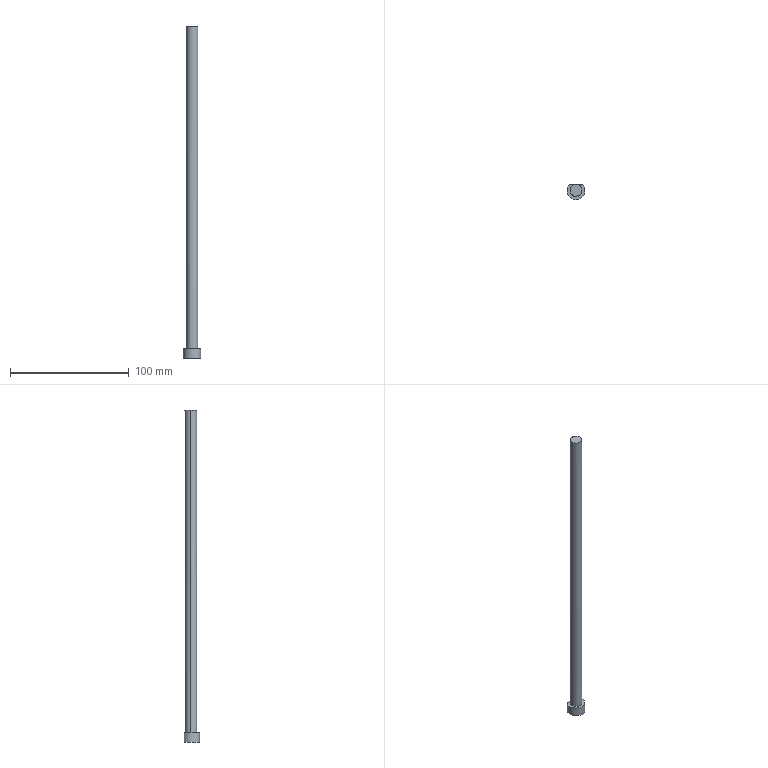Part | Creo | 1 solid | 7 faces | box 15 x 13 x 280.149 mm | volume 22672 mm3 | plane 4 | cylinder 3 | commonest cylinder face diameters 10 x2 15 x1
STEP:
#1=CARTESIAN_POINT('',(0.,0.,0.));
#2=DIRECTION('',(0.,0.,1.));
#3=DIRECTION('',(1.,0.,0.));
#4=AXIS2_PLACEMENT_3D('',#1,#2,#3);
#5=CARTESIAN_POINT('',(82.241,-116.919,-330.441));
#6=VERTEX_POINT('',#5);
#7=CARTESIAN_POINT('',(72.043,-116.919,-330.441));
#8=VERTEX_POINT('',#7);
#9=CARTESIAN_POINT('',(82.241,-116.919,-330.441));
#10=DIRECTION('',(-1.,0.,0.));
#11=VECTOR('',#10,10.198);
#12=LINE('',#9,#11);
#13=EDGE_CURVE('',#6,#8,#12,.T.);
#14=ORIENTED_EDGE('',*,*,#13,.F.);
#15=CARTESIAN_POINT('',(77.142,-122.419,-330.441));
#16=DIRECTION('',(0.,0.,-1.));
#17=DIRECTION('',(0.6799,0.7333,0.));
#18=AXIS2_PLACEMENT_3D('',#15,#16,#17);
#19=CIRCLE('',#18,7.5);
#20=EDGE_CURVE('',#6,#8,#19,.T.);
#21=ORIENTED_EDGE('',*,*,#20,.T.);
#22=EDGE_LOOP('',(#14,#21));
#23=FACE_OUTER_BOUND('',#22,.F.);
#24=CARTESIAN_POINT('',(72.142,-122.419,-330.441));
#25=VERTEX_POINT('',#24);
#26=CARTESIAN_POINT('',(82.142,-122.419,-330.441));
#27=VERTEX_POINT('',#26);
#28=CARTESIAN_POINT('',(77.142,-122.419,-330.441));
#29=DIRECTION('',(0.,0.,-1.));
#30=DIRECTION('',(-1.,0.,0.));
#31=AXIS2_PLACEMENT_3D('',#28,#29,#30);
#32=CIRCLE('',#31,5.);
#33=EDGE_CURVE('',#25,#27,#32,.T.);
#34=ORIENTED_EDGE('',*,*,#33,.F.);
#35=CARTESIAN_POINT('',(77.142,-122.419,-330.441));
#36=DIRECTION('',(0.,0.,-1.));
#37=DIRECTION('',(1.,0.,0.));
#38=AXIS2_PLACEMENT_3D('',#35,#36,#37);
#39=CIRCLE('',#38,5.);
#40=EDGE_CURVE('',#27,#25,#39,.T.);
#41=ORIENTED_EDGE('',*,*,#40,.F.);
#42=EDGE_LOOP('',(#34,#41));
#43=FACE_BOUND('',#42,.F.);
#44=CARTESIAN_POINT('',(77.142,-122.419,-330.441));
#45=DIRECTION('',(0.,0.,-1.));
#46=DIRECTION('',(-1.,0.,0.));
#47=AXIS2_PLACEMENT_3D('',#44,#45,#46);
#48=PLANE('',#47);
#49=ADVANCED_FACE('',(#23,#43),#48,.F.);
#50=CARTESIAN_POINT('',(82.142,-122.419,-58.357));
#51=VERTEX_POINT('',#50);
#52=CARTESIAN_POINT('',(77.471,-117.43,-58.293));
#53=VERTEX_POINT('',#52);
#54=CARTESIAN_POINT('',(82.142,-122.419,-58.357));
#55=CARTESIAN_POINT('',(82.142,-121.639,-58.346));
#56=CARTESIAN_POINT('',(81.818,-120.381,-58.329));
#57=CARTESIAN_POINT('',(80.863,-118.936,-58.31));
#58=CARTESIAN_POINT('',(79.483,-117.887,-58.297));
#59=CARTESIAN_POINT('',(78.25,-117.481,-58.293));
#60=B_SPLINE_CURVE_WITH_KNOTS('',3,(#54,#55,#56,#57,#58,#59,#52),.UNSPECIFIED.,.F.,.F.,(4,1,1,1,4),(0.,0.25,0.5,0.75,1.),.UNSPECIFIED.);
#61=EDGE_CURVE('',#51,#53,#60,.T.);
#62=ORIENTED_EDGE('',*,*,#61,.T.);
#63=CARTESIAN_POINT('',(72.142,-122.419,-58.366));
#64=VERTEX_POINT('',#63);
#65=CARTESIAN_POINT('',(77.471,-117.43,-58.293));
#66=CARTESIAN_POINT('',(76.583,-117.371,-58.293));
#67=CARTESIAN_POINT('',(75.21,-117.684,-58.298));
#68=CARTESIAN_POINT('',(73.648,-118.687,-58.314));
#69=CARTESIAN_POINT('',(72.545,-120.179,-58.335));
#70=CARTESIAN_POINT('',(72.142,-121.528,-58.354));
#71=CARTESIAN_POINT('',(72.142,-122.419,-58.366));
#72=B_SPLINE_CURVE_WITH_KNOTS('',3,(#65,#66,#67,#68,#69,#70,#71),.UNSPECIFIED.,.F.,.F.,(4,1,1,1,4),(0.,0.25,0.5,0.75,1.),.UNSPECIFIED.);
#73=EDGE_CURVE('',#53,#64,#72,.T.);
#74=ORIENTED_EDGE('',*,*,#73,.T.);
#75=CARTESIAN_POINT('',(72.142,-122.419,-330.441));
#76=DIRECTION('',(0.,0.,1.));
#77=VECTOR('',#76,272.075);
#78=LINE('',#75,#77);
#79=EDGE_CURVE('',#25,#64,#78,.T.);
#80=ORIENTED_EDGE('',*,*,#79,.F.);
#81=ORIENTED_EDGE('',*,*,#33,.T.);
#82=CARTESIAN_POINT('',(82.142,-122.419,-330.441));
#83=DIRECTION('',(0.,0.,1.));
#84=VECTOR('',#83,272.084);
#85=LINE('',#82,#84);
#86=EDGE_CURVE('',#27,#51,#85,.T.);
#87=ORIENTED_EDGE('',*,*,#86,.T.);
#88=EDGE_LOOP('',(#62,#74,#80,#81,#87));
#89=FACE_OUTER_BOUND('',#88,.F.);
#90=CARTESIAN_POINT('',(77.142,-122.419,-653.441));
#91=DIRECTION('',(0.,0.,1.));
#92=DIRECTION('',(1.,0.,0.));
#93=AXIS2_PLACEMENT_3D('',#90,#91,#92);
#94=CYLINDRICAL_SURFACE('',#93,5.);
#95=ADVANCED_FACE('',(#89),#94,.T.);
#96=ORIENTED_EDGE('',*,*,#73,.F.);
#97=ORIENTED_EDGE('',*,*,#61,.F.);
#98=CARTESIAN_POINT('',(72.142,-122.419,-58.366));
#99=CARTESIAN_POINT('',(72.142,-123.008,-58.374));
#100=CARTESIAN_POINT('',(72.356,-124.281,-58.391));
#101=CARTESIAN_POINT('',(73.497,-126.06,-58.415));
#102=CARTESIAN_POINT('',(75.292,-127.205,-58.429));
#103=CARTESIAN_POINT('',(77.142,-127.525,-58.432));
#104=CARTESIAN_POINT('',(78.991,-127.205,-58.426));
#105=CARTESIAN_POINT('',(80.786,-126.06,-58.408));
#106=CARTESIAN_POINT('',(81.927,-124.281,-58.383));
#107=CARTESIAN_POINT('',(82.142,-123.008,-58.365));
#108=CARTESIAN_POINT('',(82.142,-122.419,-58.357));
#109=B_SPLINE_CURVE_WITH_KNOTS('',3,(#98,#99,#100,#101,#102,#103,#104,#105,#106,#107,#108),.UNSPECIFIED.,.F.,.F.,(4,1,1,1,1,1,1,1,4),(0.,0.125,0.25,0.375,0.5,0.625,0.75,0.875,1.),.UNSPECIFIED.);
#110=EDGE_CURVE('',#64,#51,#109,.T.);
#111=ORIENTED_EDGE('',*,*,#110,.F.);
#112=EDGE_LOOP('',(#96,#97,#111));
#113=FACE_OUTER_BOUND('',#112,.F.);
#114=CARTESIAN_POINT('',(138.548,-96.213,-57.947));
#115=DIRECTION('',(0.0009059,0.01371,-0.9999));
#116=DIRECTION('',(0.,0.9999,0.01371));
#117=AXIS2_PLACEMENT_3D('',#114,#115,#116);
#118=PLANE('',#117);
#119=ADVANCED_FACE('',(#113),#118,.F.);
#120=ORIENTED_EDGE('',*,*,#110,.T.);
#121=ORIENTED_EDGE('',*,*,#86,.F.);
#122=ORIENTED_EDGE('',*,*,#40,.T.);
#123=ORIENTED_EDGE('',*,*,#79,.T.);
#124=EDGE_LOOP('',(#120,#121,#122,#123));
#125=FACE_OUTER_BOUND('',#124,.F.);
#126=CARTESIAN_POINT('',(77.142,-122.419,-653.441));
#127=DIRECTION('',(0.,0.,1.));
#128=DIRECTION('',(1.,0.,0.));
#129=AXIS2_PLACEMENT_3D('',#126,#127,#128);
#130=CYLINDRICAL_SURFACE('',#129,5.);
#131=ADVANCED_FACE('',(#125),#130,.T.);
#132=CARTESIAN_POINT('',(72.043,-116.919,-338.441));
#133=VERTEX_POINT('',#132);
#134=CARTESIAN_POINT('',(72.043,-116.919,-330.441));
#135=DIRECTION('',(0.,0.,-1.));
#136=VECTOR('',#135,8.);
#137=LINE('',#134,#136);
#138=EDGE_CURVE('',#8,#133,#137,.T.);
#139=ORIENTED_EDGE('',*,*,#138,.T.);
#140=CARTESIAN_POINT('',(82.241,-116.919,-338.441));
#141=VERTEX_POINT('',#140);
#142=CARTESIAN_POINT('',(82.241,-116.919,-338.441));
#143=DIRECTION('',(-1.,0.,0.));
#144=VECTOR('',#143,10.198);
#145=LINE('',#142,#144);
#146=EDGE_CURVE('',#141,#133,#145,.T.);
#147=ORIENTED_EDGE('',*,*,#146,.F.);
#148=CARTESIAN_POINT('',(82.241,-116.919,-338.441));
#149=DIRECTION('',(0.,0.,1.));
#150=VECTOR('',#149,8.);
#151=LINE('',#148,#150);
#152=EDGE_CURVE('',#141,#6,#151,.T.);
#153=ORIENTED_EDGE('',*,*,#152,.T.);
#154=ORIENTED_EDGE('',*,*,#13,.T.);
#155=EDGE_LOOP('',(#139,#147,#153,#154));
#156=FACE_OUTER_BOUND('',#155,.F.);
#157=CARTESIAN_POINT('',(77.142,-116.919,-338.441));
#158=DIRECTION('',(0.,1.,0.));
#159=DIRECTION('',(0.,0.,1.));
#160=AXIS2_PLACEMENT_3D('',#157,#158,#159);
#161=PLANE('',#160);
#162=ADVANCED_FACE('',(#156),#161,.T.);
#163=CARTESIAN_POINT('',(77.142,-122.419,-338.441));
#164=DIRECTION('',(0.,0.,1.));
#165=DIRECTION('',(-0.6799,0.7333,0.));
#166=AXIS2_PLACEMENT_3D('',#163,#164,#165);
#167=CIRCLE('',#166,7.5);
#168=EDGE_CURVE('',#133,#141,#167,.T.);
#169=ORIENTED_EDGE('',*,*,#168,.F.);
#170=ORIENTED_EDGE('',*,*,#138,.F.);
#171=ORIENTED_EDGE('',*,*,#20,.F.);
#172=ORIENTED_EDGE('',*,*,#152,.F.);
#173=EDGE_LOOP('',(#169,#170,#171,#172));
#174=FACE_OUTER_BOUND('',#173,.F.);
#175=CARTESIAN_POINT('',(77.142,-122.419,-330.441));
#176=DIRECTION('',(0.,0.,-1.));
#177=DIRECTION('',(-1.,0.,0.));
#178=AXIS2_PLACEMENT_3D('',#175,#176,#177);
#179=CYLINDRICAL_SURFACE('',#178,7.5);
#180=ADVANCED_FACE('',(#174),#179,.T.);
#181=ORIENTED_EDGE('',*,*,#168,.T.);
#182=ORIENTED_EDGE('',*,*,#146,.T.);
#183=EDGE_LOOP('',(#181,#182));
#184=FACE_OUTER_BOUND('',#183,.F.);
#185=CARTESIAN_POINT('',(77.142,-122.419,-338.441));
#186=DIRECTION('',(0.,0.,-1.));
#187=DIRECTION('',(-1.,0.,0.));
#188=AXIS2_PLACEMENT_3D('',#185,#186,#187);
#189=PLANE('',#188);
#190=ADVANCED_FACE('',(#184),#189,.T.);
#191=CLOSED_SHELL('',(#49,#95,#119,#131,#162,#180,#190));
#192=MANIFOLD_SOLID_BREP('',#191);
#193=(LENGTH_UNIT()NAMED_UNIT(*)SI_UNIT(.MILLI.,.METRE.));
#194=UNCERTAINTY_MEASURE_WITH_UNIT(LENGTH_MEASURE(0.02808),#193,'','');
#195=(NAMED_UNIT(*)PLANE_ANGLE_UNIT()SI_UNIT($,.RADIAN.));
#196=PLANE_ANGLE_MEASURE_WITH_UNIT(PLANE_ANGLE_MEASURE(0.01745),#195);
#197=(CONVERSION_BASED_UNIT('DEGREE',#196)NAMED_UNIT(*)PLANE_ANGLE_UNIT());
#198=(NAMED_UNIT(*)SI_UNIT($,.STERADIAN.)SOLID_ANGLE_UNIT());
#199=(GEOMETRIC_REPRESENTATION_CONTEXT(3)GLOBAL_UNCERTAINTY_ASSIGNED_CONTEXT((#194))GLOBAL_UNIT_ASSIGNED_CONTEXT((#193,#197,#198))REPRESENTATION_CONTEXT('',''));
#200=ADVANCED_BREP_SHAPE_REPRESENTATION('',(#4,#192),#199);